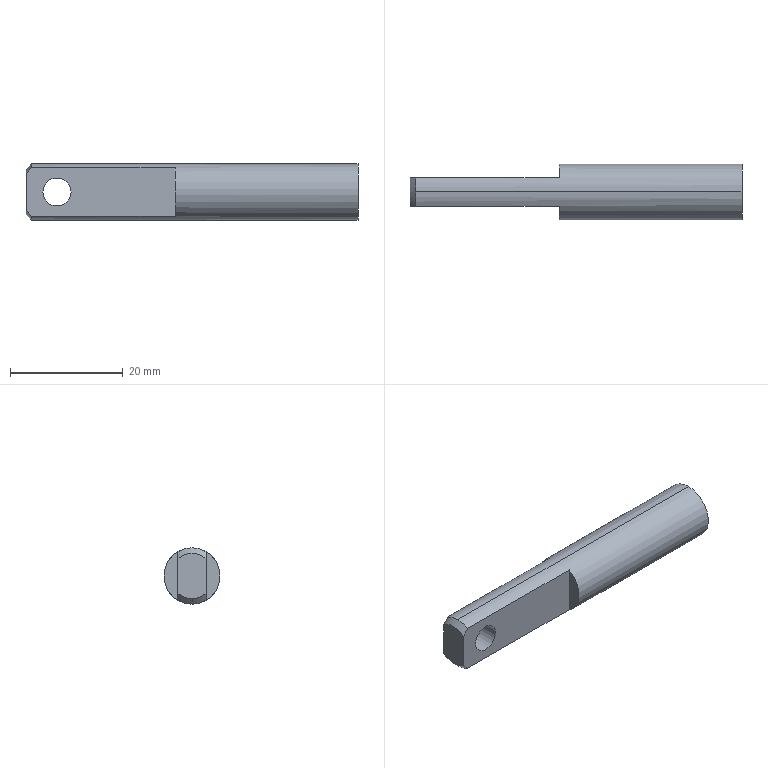Part | STEP file | mandrel_default | 1 solid | 13 faces | box 59 x 10 x 10 mm | volume 3717 mm3 | plane 6 | cylinder 4 | cone 3 | commonest cylinder face diameters 5 x2 10 x2
STEP:
#1=CARTESIAN_POINT('',(0.,0.,0.));
#2=DIRECTION('',(0.,0.,1.));
#3=DIRECTION('',(1.,0.,0.));
#4=AXIS2_PLACEMENT_3D('',#1,#2,#3);
#5=CARTESIAN_POINT('',(-59.,0.,-4.));
#6=VERTEX_POINT('',#5);
#7=CARTESIAN_POINT('',(-59.,-2.5,-3.122));
#8=VERTEX_POINT('',#7);
#9=CARTESIAN_POINT('',(-59.,0.,0.));
#10=DIRECTION('',(-1.,0.,0.));
#11=DIRECTION('',(0.,0.,-1.));
#12=AXIS2_PLACEMENT_3D('',#9,#10,#11);
#13=CIRCLE('',#12,4.);
#14=CARTESIAN_POINT('',(-58.,0.,0.));
#15=DIRECTION('',(1.,0.,0.));
#16=DIRECTION('',(0.,0.,-1.));
#17=AXIS2_PLACEMENT_3D('',#14,#15,#16);
#18=CONICAL_SURFACE('',#17,5.,0.7854);
#19=CARTESIAN_POINT('',(6.283,-1.));
#20=DIRECTION('',(-1.,0.));
#21=VECTOR('',#20,1.);
#22=LINE('',#19,#21);
#23=(GEOMETRIC_REPRESENTATION_CONTEXT(2)PARAMETRIC_REPRESENTATION_CONTEXT()REPRESENTATION_CONTEXT('',''));
#24=DEFINITIONAL_REPRESENTATION('',(#22),#23);
#25=PCURVE('',#18,#24);
#26=CARTESIAN_POINT('',(-59.,0.,0.));
#27=DIRECTION('',(1.,0.,0.));
#28=DIRECTION('',(0.,0.,-1.));
#29=AXIS2_PLACEMENT_3D('',#26,#27,#28);
#30=PLANE('',#29);
#31=CARTESIAN_POINT('',(4.,0.));
#32=CARTESIAN_POINT('',(4.,-6.928));
#33=CARTESIAN_POINT('',(-2.,-3.464));
#34=CARTESIAN_POINT('',(-8.,0.));
#35=CARTESIAN_POINT('',(-2.,3.464));
#36=CARTESIAN_POINT('',(4.,6.928));
#37=CARTESIAN_POINT('',(4.,0.));
#38=(BOUNDED_CURVE()B_SPLINE_CURVE(2,(#31,#32,#33,#34,#35,#36,#37),.UNSPECIFIED.,.T.,.F.)B_SPLINE_CURVE_WITH_KNOTS((1,2,2,2,2,1),(-2.094,0.,2.094,4.189,6.283,8.378),.UNSPECIFIED.)CURVE()GEOMETRIC_REPRESENTATION_ITEM()RATIONAL_B_SPLINE_CURVE((1.,0.5,1.,0.5,1.,0.5,1.))REPRESENTATION_ITEM(''));
#39=(GEOMETRIC_REPRESENTATION_CONTEXT(2)PARAMETRIC_REPRESENTATION_CONTEXT()REPRESENTATION_CONTEXT('',''));
#40=DEFINITIONAL_REPRESENTATION('',(#38),#39);
#41=PCURVE('',#30,#40);
#42=SURFACE_CURVE('',#13,(#25,#41),.PCURVE_S1.);
#43=EDGE_CURVE('',#6,#8,#42,.T.);
#44=ORIENTED_EDGE('',*,*,#43,.F.);
#45=CARTESIAN_POINT('',(-58.,0.,-5.));
#46=VERTEX_POINT('',#45);
#47=CARTESIAN_POINT('',(-58.,0.,-5.));
#48=DIRECTION('',(0.7071,0.,-0.7071));
#49=VECTOR('',#48,1.);
#50=LINE('',#47,#49);
#51=CARTESIAN_POINT('',(6.283,0.));
#52=DIRECTION('',(0.,1.));
#53=VECTOR('',#52,1.);
#54=LINE('',#51,#53);
#55=(GEOMETRIC_REPRESENTATION_CONTEXT(2)PARAMETRIC_REPRESENTATION_CONTEXT()REPRESENTATION_CONTEXT('',''));
#56=DEFINITIONAL_REPRESENTATION('',(#54),#55);
#57=PCURVE('',#18,#56);
#58=CARTESIAN_POINT('',(-58.,0.,0.));
#59=DIRECTION('',(1.,0.,0.));
#60=DIRECTION('',(0.,0.,-1.));
#61=AXIS2_PLACEMENT_3D('',#58,#59,#60);
#62=CONICAL_SURFACE('',#61,5.,0.7854);
#63=CARTESIAN_POINT('',(0.,0.));
#64=DIRECTION('',(0.,1.));
#65=VECTOR('',#64,1.);
#66=LINE('',#63,#65);
#67=(GEOMETRIC_REPRESENTATION_CONTEXT(2)PARAMETRIC_REPRESENTATION_CONTEXT()REPRESENTATION_CONTEXT('',''));
#68=DEFINITIONAL_REPRESENTATION('',(#66),#67);
#69=PCURVE('',#62,#68);
#70=SURFACE_CURVE('',#50,(#57,#69),.PCURVE_S1.);
#71=EDGE_CURVE('',#6,#46,#70,.T.);
#72=ORIENTED_EDGE('',*,*,#71,.T.);
#73=CARTESIAN_POINT('',(-58.,-2.5,-4.33));
#74=VERTEX_POINT('',#73);
#75=CARTESIAN_POINT('',(-58.,0.,0.));
#76=DIRECTION('',(1.,0.,0.));
#77=DIRECTION('',(0.,0.,-1.));
#78=AXIS2_PLACEMENT_3D('',#75,#76,#77);
#79=CIRCLE('',#78,5.);
#80=CARTESIAN_POINT('',(0.,0.));
#81=DIRECTION('',(1.,0.));
#82=VECTOR('',#81,1.);
#83=LINE('',#80,#82);
#84=(GEOMETRIC_REPRESENTATION_CONTEXT(2)PARAMETRIC_REPRESENTATION_CONTEXT()REPRESENTATION_CONTEXT('',''));
#85=DEFINITIONAL_REPRESENTATION('',(#83),#84);
#86=PCURVE('',#18,#85);
#87=CARTESIAN_POINT('',(-59.,0.,0.));
#88=DIRECTION('',(1.,0.,0.));
#89=DIRECTION('',(0.,0.,-1.));
#90=AXIS2_PLACEMENT_3D('',#87,#88,#89);
#91=CYLINDRICAL_SURFACE('',#90,5.);
#92=CARTESIAN_POINT('',(0.,1.));
#93=DIRECTION('',(1.,0.));
#94=VECTOR('',#93,1.);
#95=LINE('',#92,#94);
#96=(GEOMETRIC_REPRESENTATION_CONTEXT(2)PARAMETRIC_REPRESENTATION_CONTEXT()REPRESENTATION_CONTEXT('',''));
#97=DEFINITIONAL_REPRESENTATION('',(#95),#96);
#98=PCURVE('',#91,#97);
#99=SURFACE_CURVE('',#79,(#86,#98),.PCURVE_S1.);
#100=EDGE_CURVE('',#74,#46,#99,.T.);
#101=ORIENTED_EDGE('',*,*,#100,.F.);
#102=CARTESIAN_POINT('',(-59.,-2.5,-3.122));
#103=CARTESIAN_POINT('',(-58.678,-2.5,-3.535));
#104=CARTESIAN_POINT('',(-58.342,-2.5,-3.935));
#105=CARTESIAN_POINT('',(-58.,-2.5,-4.33));
#106=B_SPLINE_CURVE_WITH_KNOTS('',3,(#102,#103,#104,#105),.UNSPECIFIED.,.F.,.F.,(4,4),(0.,0.001568),.PIECEWISE_BEZIER_KNOTS.);
#107=CARTESIAN_POINT('',(5.608,-1.));
#108=CARTESIAN_POINT('',(5.611,-0.9854));
#109=CARTESIAN_POINT('',(5.617,-0.9561));
#110=CARTESIAN_POINT('',(5.625,-0.9119));
#111=CARTESIAN_POINT('',(5.633,-0.8676));
#112=CARTESIAN_POINT('',(5.642,-0.8231));
#113=CARTESIAN_POINT('',(5.649,-0.7785));
#114=CARTESIAN_POINT('',(5.657,-0.7337));
#115=CARTESIAN_POINT('',(5.665,-0.6887));
#116=CARTESIAN_POINT('',(5.672,-0.6437));
#117=CARTESIAN_POINT('',(5.679,-0.5984));
#118=CARTESIAN_POINT('',(5.686,-0.5531));
#119=CARTESIAN_POINT('',(5.693,-0.5076));
#120=CARTESIAN_POINT('',(5.7,-0.462));
#121=CARTESIAN_POINT('',(5.706,-0.4163));
#122=CARTESIAN_POINT('',(5.713,-0.3704));
#123=CARTESIAN_POINT('',(5.719,-0.3245));
#124=CARTESIAN_POINT('',(5.725,-0.2784));
#125=CARTESIAN_POINT('',(5.731,-0.2322));
#126=CARTESIAN_POINT('',(5.737,-0.186));
#127=CARTESIAN_POINT('',(5.743,-0.1396));
#128=CARTESIAN_POINT('',(5.749,-0.09318));
#129=CARTESIAN_POINT('',(5.754,-0.04664));
#130=CARTESIAN_POINT('',(5.758,-0.01556));
#131=CARTESIAN_POINT('',(5.76,0.));
#132=B_SPLINE_CURVE_WITH_KNOTS('',3,(#107,#108,#109,#110,#111,#112,#113,#114,#115,#116,#117,#118,#119,#120,#121,#122,#123,#124,#125,#126,#127,#128,#129,#130,#131),.UNSPECIFIED.,.F.,.F.,(4,1,1,1,1,1,1,1,1,1,1,1,1,1,1,1,1,1,1,1,1,1,4),(0.,0.00007127,0.0001425,0.0002138,0.0002851,0.0003563,0.0004276,0.0004989,0.0005702,0.0006414,0.0007127,0.000784,0.0008552,0.0009265,0.0009978,0.001069,0.00114,0.001212,0.001283,0.001354,0.001425,0.001497,0.001568),.QUASI_UNIFORM_KNOTS.);
#133=(GEOMETRIC_REPRESENTATION_CONTEXT(2)PARAMETRIC_REPRESENTATION_CONTEXT()REPRESENTATION_CONTEXT('',''));
#134=DEFINITIONAL_REPRESENTATION('',(#132),#133);
#135=PCURVE('',#18,#134);
#136=CARTESIAN_POINT('',(-64.008,-2.5,-5.));
#137=DIRECTION('',(0.,1.,0.));
#138=DIRECTION('',(-1.,0.,0.));
#139=AXIS2_PLACEMENT_3D('',#136,#137,#138);
#140=PLANE('',#139);
#141=CARTESIAN_POINT('',(-5.008,1.878));
#142=CARTESIAN_POINT('',(-5.33,1.465));
#143=CARTESIAN_POINT('',(-5.666,1.065));
#144=CARTESIAN_POINT('',(-6.008,0.6699));
#145=B_SPLINE_CURVE_WITH_KNOTS('',3,(#141,#142,#143,#144),.UNSPECIFIED.,.F.,.F.,(4,4),(0.,0.001568),.PIECEWISE_BEZIER_KNOTS.);
#146=(GEOMETRIC_REPRESENTATION_CONTEXT(2)PARAMETRIC_REPRESENTATION_CONTEXT()REPRESENTATION_CONTEXT('',''));
#147=DEFINITIONAL_REPRESENTATION('',(#145),#146);
#148=PCURVE('',#140,#147);
#149=SURFACE_CURVE('',#106,(#135,#148),.PCURVE_S1.);
#150=EDGE_CURVE('',#8,#74,#149,.T.);
#151=ORIENTED_EDGE('',*,*,#150,.F.);
#152=EDGE_LOOP('',(#44,#72,#101,#151));
#153=FACE_BOUND('',#152,.T.);
#154=ADVANCED_FACE('',(#153),#18,.T.);
#155=CARTESIAN_POINT('',(-56.,-2.5,0.));
#156=VERTEX_POINT('',#155);
#157=CARTESIAN_POINT('',(-56.,2.5,0.));
#158=VERTEX_POINT('',#157);
#159=CARTESIAN_POINT('',(-56.,-5.,0.));
#160=DIRECTION('',(0.,1.,0.));
#161=VECTOR('',#160,1.);
#162=LINE('',#159,#161);
#163=CARTESIAN_POINT('',(-53.5,-5.,0.));
#164=DIRECTION('',(0.,1.,0.));
#165=DIRECTION('',(-1.,0.,0.));
#166=AXIS2_PLACEMENT_3D('',#163,#164,#165);
#167=CYLINDRICAL_SURFACE('',#166,2.5);
#168=CARTESIAN_POINT('',(6.283,0.));
#169=DIRECTION('',(0.,1.));
#170=VECTOR('',#169,1.);
#171=LINE('',#168,#170);
#172=(GEOMETRIC_REPRESENTATION_CONTEXT(2)PARAMETRIC_REPRESENTATION_CONTEXT()REPRESENTATION_CONTEXT('',''));
#173=DEFINITIONAL_REPRESENTATION('',(#171),#172);
#174=PCURVE('',#167,#173);
#175=CARTESIAN_POINT('',(-53.5,-5.,0.));
#176=DIRECTION('',(0.,1.,0.));
#177=DIRECTION('',(-1.,0.,0.));
#178=AXIS2_PLACEMENT_3D('',#175,#176,#177);
#179=CYLINDRICAL_SURFACE('',#178,2.5);
#180=CARTESIAN_POINT('',(0.,0.));
#181=DIRECTION('',(0.,1.));
#182=VECTOR('',#181,1.);
#183=LINE('',#180,#182);
#184=(GEOMETRIC_REPRESENTATION_CONTEXT(2)PARAMETRIC_REPRESENTATION_CONTEXT()REPRESENTATION_CONTEXT('',''));
#185=DEFINITIONAL_REPRESENTATION('',(#183),#184);
#186=PCURVE('',#179,#185);
#187=SURFACE_CURVE('',#162,(#174,#186),.PCURVE_S1.);
#188=EDGE_CURVE('',#156,#158,#187,.T.);
#189=ORIENTED_EDGE('',*,*,#188,.T.);
#190=CARTESIAN_POINT('',(-51.,2.5,0.));
#191=VERTEX_POINT('',#190);
#192=CARTESIAN_POINT('',(-53.5,2.5,0.));
#193=DIRECTION('',(0.,1.,0.));
#194=DIRECTION('',(-1.,0.,0.));
#195=AXIS2_PLACEMENT_3D('',#192,#193,#194);
#196=CIRCLE('',#195,2.5);
#197=CARTESIAN_POINT('',(0.,7.5));
#198=DIRECTION('',(1.,0.));
#199=VECTOR('',#198,1.);
#200=LINE('',#197,#199);
#201=(GEOMETRIC_REPRESENTATION_CONTEXT(2)PARAMETRIC_REPRESENTATION_CONTEXT()REPRESENTATION_CONTEXT('',''));
#202=DEFINITIONAL_REPRESENTATION('',(#200),#201);
#203=PCURVE('',#167,#202);
#204=CARTESIAN_POINT('',(-61.463,2.5,-5.));
#205=DIRECTION('',(0.,-1.,0.));
#206=DIRECTION('',(1.,0.,0.));
#207=AXIS2_PLACEMENT_3D('',#204,#205,#206);
#208=PLANE('',#207);
#209=CARTESIAN_POINT('',(5.463,5.));
#210=CARTESIAN_POINT('',(5.463,9.33));
#211=CARTESIAN_POINT('',(9.213,7.165));
#212=CARTESIAN_POINT('',(12.963,5.));
#213=CARTESIAN_POINT('',(9.213,2.835));
#214=CARTESIAN_POINT('',(5.463,0.6699));
#215=CARTESIAN_POINT('',(5.463,5.));
#216=(BOUNDED_CURVE()B_SPLINE_CURVE(2,(#209,#210,#211,#212,#213,#214,#215),.UNSPECIFIED.,.T.,.F.)B_SPLINE_CURVE_WITH_KNOTS((1,2,2,2,2,1),(-2.094,0.,2.094,4.189,6.283,8.378),.UNSPECIFIED.)CURVE()GEOMETRIC_REPRESENTATION_ITEM()RATIONAL_B_SPLINE_CURVE((1.,0.5,1.,0.5,1.,0.5,1.))REPRESENTATION_ITEM(''));
#217=(GEOMETRIC_REPRESENTATION_CONTEXT(2)PARAMETRIC_REPRESENTATION_CONTEXT()REPRESENTATION_CONTEXT('',''));
#218=DEFINITIONAL_REPRESENTATION('',(#216),#217);
#219=PCURVE('',#208,#218);
#220=SURFACE_CURVE('',#196,(#203,#219),.PCURVE_S1.);
#221=EDGE_CURVE('',#191,#158,#220,.T.);
#222=ORIENTED_EDGE('',*,*,#221,.F.);
#223=CARTESIAN_POINT('',(-51.,-2.5,0.));
#224=VERTEX_POINT('',#223);
#225=CARTESIAN_POINT('',(-51.,-5.,0.));
#226=DIRECTION('',(0.,1.,0.));
#227=VECTOR('',#226,1.);
#228=LINE('',#225,#227);
#229=CARTESIAN_POINT('',(3.142,0.));
#230=DIRECTION('',(0.,1.));
#231=VECTOR('',#230,1.);
#232=LINE('',#229,#231);
#233=(GEOMETRIC_REPRESENTATION_CONTEXT(2)PARAMETRIC_REPRESENTATION_CONTEXT()REPRESENTATION_CONTEXT('',''));
#234=DEFINITIONAL_REPRESENTATION('',(#232),#233);
#235=PCURVE('',#167,#234);
#236=CARTESIAN_POINT('',(3.142,0.));
#237=DIRECTION('',(0.,1.));
#238=VECTOR('',#237,1.);
#239=LINE('',#236,#238);
#240=(GEOMETRIC_REPRESENTATION_CONTEXT(2)PARAMETRIC_REPRESENTATION_CONTEXT()REPRESENTATION_CONTEXT('',''));
#241=DEFINITIONAL_REPRESENTATION('',(#239),#240);
#242=PCURVE('',#179,#241);
#243=SURFACE_CURVE('',#228,(#235,#242),.PCURVE_S1.);
#244=EDGE_CURVE('',#224,#191,#243,.T.);
#245=ORIENTED_EDGE('',*,*,#244,.F.);
#246=CARTESIAN_POINT('',(-53.5,-2.5,0.));
#247=DIRECTION('',(0.,1.,0.));
#248=DIRECTION('',(-1.,0.,0.));
#249=AXIS2_PLACEMENT_3D('',#246,#247,#248);
#250=CIRCLE('',#249,2.5);
#251=CARTESIAN_POINT('',(0.,2.5));
#252=DIRECTION('',(1.,0.));
#253=VECTOR('',#252,1.);
#254=LINE('',#251,#253);
#255=(GEOMETRIC_REPRESENTATION_CONTEXT(2)PARAMETRIC_REPRESENTATION_CONTEXT()REPRESENTATION_CONTEXT('',''));
#256=DEFINITIONAL_REPRESENTATION('',(#254),#255);
#257=PCURVE('',#167,#256);
#258=CARTESIAN_POINT('',(-10.508,5.));
#259=DIRECTION('',(1.,0.));
#260=AXIS2_PLACEMENT_2D('',#258,#259);
#261=CIRCLE('',#260,2.5);
#262=(GEOMETRIC_REPRESENTATION_CONTEXT(2)PARAMETRIC_REPRESENTATION_CONTEXT()REPRESENTATION_CONTEXT('',''));
#263=DEFINITIONAL_REPRESENTATION('',(#261),#262);
#264=PCURVE('',#140,#263);
#265=SURFACE_CURVE('',#250,(#257,#264),.PCURVE_S1.);
#266=EDGE_CURVE('',#224,#156,#265,.T.);
#267=ORIENTED_EDGE('',*,*,#266,.T.);
#268=EDGE_LOOP('',(#189,#222,#245,#267));
#269=FACE_BOUND('',#268,.F.);
#270=ADVANCED_FACE('',(#269),#167,.F.);
#271=CARTESIAN_POINT('',(-58.,2.5,4.33));
#272=VERTEX_POINT('',#271);
#273=CARTESIAN_POINT('',(-58.,0.,5.));
#274=VERTEX_POINT('',#273);
#275=CARTESIAN_POINT('',(-58.,0.,0.));
#276=DIRECTION('',(1.,0.,0.));
#277=DIRECTION('',(0.,0.,-1.));
#278=AXIS2_PLACEMENT_3D('',#275,#276,#277);
#279=CIRCLE('',#278,5.);
#280=CARTESIAN_POINT('',(-59.,0.,0.));
#281=DIRECTION('',(1.,0.,0.));
#282=DIRECTION('',(0.,0.,-1.));
#283=AXIS2_PLACEMENT_3D('',#280,#281,#282);
#284=CYLINDRICAL_SURFACE('',#283,5.);
#285=CARTESIAN_POINT('',(0.,1.));
#286=DIRECTION('',(1.,0.));
#287=VECTOR('',#286,1.);
#288=LINE('',#285,#287);
#289=(GEOMETRIC_REPRESENTATION_CONTEXT(2)PARAMETRIC_REPRESENTATION_CONTEXT()REPRESENTATION_CONTEXT('',''));
#290=DEFINITIONAL_REPRESENTATION('',(#288),#289);
#291=PCURVE('',#284,#290);
#292=CARTESIAN_POINT('',(-58.,0.,0.));
#293=DIRECTION('',(1.,0.,0.));
#294=DIRECTION('',(0.,0.,-1.));
#295=AXIS2_PLACEMENT_3D('',#292,#293,#294);
#296=CONICAL_SURFACE('',#295,5.,0.7854);
#297=CARTESIAN_POINT('',(0.,0.));
#298=DIRECTION('',(1.,0.));
#299=VECTOR('',#298,1.);
#300=LINE('',#297,#299);
#301=(GEOMETRIC_REPRESENTATION_CONTEXT(2)PARAMETRIC_REPRESENTATION_CONTEXT()REPRESENTATION_CONTEXT('',''));
#302=DEFINITIONAL_REPRESENTATION('',(#300),#301);
#303=PCURVE('',#296,#302);
#304=SURFACE_CURVE('',#279,(#291,#303),.PCURVE_S1.);
#305=EDGE_CURVE('',#272,#274,#304,.T.);
#306=ORIENTED_EDGE('',*,*,#305,.T.);
#307=CARTESIAN_POINT('',(0.,0.,5.));
#308=VERTEX_POINT('',#307);
#309=CARTESIAN_POINT('',(-59.,0.,5.));
#310=DIRECTION('',(1.,0.,0.));
#311=VECTOR('',#310,1.);
#312=LINE('',#309,#311);
#313=CARTESIAN_POINT('',(3.142,0.));
#314=DIRECTION('',(0.,1.));
#315=VECTOR('',#314,1.);
#316=LINE('',#313,#315);
#317=(GEOMETRIC_REPRESENTATION_CONTEXT(2)PARAMETRIC_REPRESENTATION_CONTEXT()REPRESENTATION_CONTEXT('',''));
#318=DEFINITIONAL_REPRESENTATION('',(#316),#317);
#319=PCURVE('',#284,#318);
#320=CARTESIAN_POINT('',(3.142,0.));
#321=DIRECTION('',(0.,1.));
#322=VECTOR('',#321,1.);
#323=LINE('',#320,#322);
#324=(GEOMETRIC_REPRESENTATION_CONTEXT(2)PARAMETRIC_REPRESENTATION_CONTEXT()REPRESENTATION_CONTEXT('',''));
#325=DEFINITIONAL_REPRESENTATION('',(#323),#324);
#326=PCURVE('',#91,#325);
#327=SURFACE_CURVE('',#312,(#319,#326),.PCURVE_S1.);
#328=EDGE_CURVE('',#274,#308,#327,.T.);
#329=ORIENTED_EDGE('',*,*,#328,.T.);
#330=CARTESIAN_POINT('',(0.,0.,-5.));
#331=VERTEX_POINT('',#330);
#332=CARTESIAN_POINT('',(0.,0.,0.));
#333=DIRECTION('',(1.,0.,0.));
#334=DIRECTION('',(0.,0.,-1.));
#335=AXIS2_PLACEMENT_3D('',#332,#333,#334);
#336=CIRCLE('',#335,5.);
#337=CARTESIAN_POINT('',(0.,59.));
#338=DIRECTION('',(1.,0.));
#339=VECTOR('',#338,1.);
#340=LINE('',#337,#339);
#341=(GEOMETRIC_REPRESENTATION_CONTEXT(2)PARAMETRIC_REPRESENTATION_CONTEXT()REPRESENTATION_CONTEXT('',''));
#342=DEFINITIONAL_REPRESENTATION('',(#340),#341);
#343=PCURVE('',#284,#342);
#344=CARTESIAN_POINT('',(0.,0.,0.));
#345=DIRECTION('',(1.,0.,0.));
#346=DIRECTION('',(0.,0.,-1.));
#347=AXIS2_PLACEMENT_3D('',#344,#345,#346);
#348=PLANE('',#347);
#349=CARTESIAN_POINT('',(0.,0.));
#350=DIRECTION('',(1.,0.));
#351=AXIS2_PLACEMENT_2D('',#349,#350);
#352=CIRCLE('',#351,5.);
#353=(GEOMETRIC_REPRESENTATION_CONTEXT(2)PARAMETRIC_REPRESENTATION_CONTEXT()REPRESENTATION_CONTEXT('',''));
#354=DEFINITIONAL_REPRESENTATION('',(#352),#353);
#355=PCURVE('',#348,#354);
#356=SURFACE_CURVE('',#336,(#343,#355),.PCURVE_S1.);
#357=EDGE_CURVE('',#331,#308,#356,.T.);
#358=ORIENTED_EDGE('',*,*,#357,.F.);
#359=CARTESIAN_POINT('',(-59.,0.,-5.));
#360=DIRECTION('',(1.,0.,0.));
#361=VECTOR('',#360,1.);
#362=LINE('',#359,#361);
#363=CARTESIAN_POINT('',(0.,0.));
#364=DIRECTION('',(0.,1.));
#365=VECTOR('',#364,1.);
#366=LINE('',#363,#365);
#367=(GEOMETRIC_REPRESENTATION_CONTEXT(2)PARAMETRIC_REPRESENTATION_CONTEXT()REPRESENTATION_CONTEXT('',''));
#368=DEFINITIONAL_REPRESENTATION('',(#366),#367);
#369=PCURVE('',#284,#368);
#370=CARTESIAN_POINT('',(6.283,0.));
#371=DIRECTION('',(0.,1.));
#372=VECTOR('',#371,1.);
#373=LINE('',#370,#372);
#374=(GEOMETRIC_REPRESENTATION_CONTEXT(2)PARAMETRIC_REPRESENTATION_CONTEXT()REPRESENTATION_CONTEXT('',''));
#375=DEFINITIONAL_REPRESENTATION('',(#373),#374);
#376=PCURVE('',#91,#375);
#377=SURFACE_CURVE('',#362,(#369,#376),.PCURVE_S1.);
#378=EDGE_CURVE('',#46,#331,#377,.T.);
#379=ORIENTED_EDGE('',*,*,#378,.F.);
#380=CARTESIAN_POINT('',(-58.,2.5,-4.33));
#381=VERTEX_POINT('',#380);
#382=CARTESIAN_POINT('',(-58.,0.,0.));
#383=DIRECTION('',(1.,0.,0.));
#384=DIRECTION('',(0.,0.,-1.));
#385=AXIS2_PLACEMENT_3D('',#382,#383,#384);
#386=CIRCLE('',#385,5.);
#387=CARTESIAN_POINT('',(0.,1.));
#388=DIRECTION('',(1.,0.));
#389=VECTOR('',#388,1.);
#390=LINE('',#387,#389);
#391=(GEOMETRIC_REPRESENTATION_CONTEXT(2)PARAMETRIC_REPRESENTATION_CONTEXT()REPRESENTATION_CONTEXT('',''));
#392=DEFINITIONAL_REPRESENTATION('',(#390),#391);
#393=PCURVE('',#284,#392);
#394=CARTESIAN_POINT('',(0.,0.));
#395=DIRECTION('',(1.,0.));
#396=VECTOR('',#395,1.);
#397=LINE('',#394,#396);
#398=(GEOMETRIC_REPRESENTATION_CONTEXT(2)PARAMETRIC_REPRESENTATION_CONTEXT()REPRESENTATION_CONTEXT('',''));
#399=DEFINITIONAL_REPRESENTATION('',(#397),#398);
#400=PCURVE('',#62,#399);
#401=SURFACE_CURVE('',#386,(#393,#400),.PCURVE_S1.);
#402=EDGE_CURVE('',#46,#381,#401,.T.);
#403=ORIENTED_EDGE('',*,*,#402,.T.);
#404=CARTESIAN_POINT('',(-32.5,2.5,-4.33));
#405=VERTEX_POINT('',#404);
#406=CARTESIAN_POINT('',(-59.,2.5,-4.33));
#407=DIRECTION('',(-1.,0.,0.));
#408=VECTOR('',#407,1.);
#409=LINE('',#406,#408);
#410=CARTESIAN_POINT('',(0.5236,0.));
#411=DIRECTION('',(0.,-1.));
#412=VECTOR('',#411,1.);
#413=LINE('',#410,#412);
#414=(GEOMETRIC_REPRESENTATION_CONTEXT(2)PARAMETRIC_REPRESENTATION_CONTEXT()REPRESENTATION_CONTEXT('',''));
#415=DEFINITIONAL_REPRESENTATION('',(#413),#414);
#416=PCURVE('',#284,#415);
#417=CARTESIAN_POINT('',(2.463,0.6699));
#418=DIRECTION('',(-1.,0.));
#419=VECTOR('',#418,1.);
#420=LINE('',#417,#419);
#421=(GEOMETRIC_REPRESENTATION_CONTEXT(2)PARAMETRIC_REPRESENTATION_CONTEXT()REPRESENTATION_CONTEXT('',''));
#422=DEFINITIONAL_REPRESENTATION('',(#420),#421);
#423=PCURVE('',#208,#422);
#424=SURFACE_CURVE('',#409,(#416,#423),.PCURVE_S1.);
#425=EDGE_CURVE('',#405,#381,#424,.T.);
#426=ORIENTED_EDGE('',*,*,#425,.F.);
#427=CARTESIAN_POINT('',(-32.5,2.5,4.33));
#428=VERTEX_POINT('',#427);
#429=CARTESIAN_POINT('',(-32.5,0.,0.));
#430=DIRECTION('',(-1.,0.,0.));
#431=DIRECTION('',(0.,0.,-1.));
#432=AXIS2_PLACEMENT_3D('',#429,#430,#431);
#433=CIRCLE('',#432,5.);
#434=CARTESIAN_POINT('',(6.283,26.5));
#435=DIRECTION('',(-1.,0.));
#436=VECTOR('',#435,1.);
#437=LINE('',#434,#436);
#438=(GEOMETRIC_REPRESENTATION_CONTEXT(2)PARAMETRIC_REPRESENTATION_CONTEXT()REPRESENTATION_CONTEXT('',''));
#439=DEFINITIONAL_REPRESENTATION('',(#437),#438);
#440=PCURVE('',#284,#439);
#441=CARTESIAN_POINT('',(-32.5,7.127,-5.));
#442=DIRECTION('',(1.,0.,0.));
#443=DIRECTION('',(0.,0.,-1.));
#444=AXIS2_PLACEMENT_3D('',#441,#442,#443);
#445=PLANE('',#444);
#446=CARTESIAN_POINT('',(0.,-7.127));
#447=CARTESIAN_POINT('',(0.,-15.787));
#448=CARTESIAN_POINT('',(-7.5,-11.457));
#449=CARTESIAN_POINT('',(-15.,-7.127));
#450=CARTESIAN_POINT('',(-7.5,-2.797));
#451=CARTESIAN_POINT('',(0.,1.533));
#452=CARTESIAN_POINT('',(0.,-7.127));
#453=(BOUNDED_CURVE()B_SPLINE_CURVE(2,(#446,#447,#448,#449,#450,#451,#452),.UNSPECIFIED.,.T.,.F.)B_SPLINE_CURVE_WITH_KNOTS((1,2,2,2,2,1),(-2.094,0.,2.094,4.189,6.283,8.378),.UNSPECIFIED.)CURVE()GEOMETRIC_REPRESENTATION_ITEM()RATIONAL_B_SPLINE_CURVE((1.,0.5,1.,0.5,1.,0.5,1.))REPRESENTATION_ITEM(''));
#454=(GEOMETRIC_REPRESENTATION_CONTEXT(2)PARAMETRIC_REPRESENTATION_CONTEXT()REPRESENTATION_CONTEXT('',''));
#455=DEFINITIONAL_REPRESENTATION('',(#453),#454);
#456=PCURVE('',#445,#455);
#457=SURFACE_CURVE('',#433,(#440,#456),.PCURVE_S1.);
#458=EDGE_CURVE('',#428,#405,#457,.T.);
#459=ORIENTED_EDGE('',*,*,#458,.F.);
#460=CARTESIAN_POINT('',(-59.,2.5,4.33));
#461=DIRECTION('',(1.,0.,0.));
#462=VECTOR('',#461,1.);
#463=LINE('',#460,#462);
#464=CARTESIAN_POINT('',(2.618,0.));
#465=DIRECTION('',(0.,1.));
#466=VECTOR('',#465,1.);
#467=LINE('',#464,#466);
#468=(GEOMETRIC_REPRESENTATION_CONTEXT(2)PARAMETRIC_REPRESENTATION_CONTEXT()REPRESENTATION_CONTEXT('',''));
#469=DEFINITIONAL_REPRESENTATION('',(#467),#468);
#470=PCURVE('',#284,#469);
#471=CARTESIAN_POINT('',(2.463,9.33));
#472=DIRECTION('',(1.,0.));
#473=VECTOR('',#472,1.);
#474=LINE('',#471,#473);
#475=(GEOMETRIC_REPRESENTATION_CONTEXT(2)PARAMETRIC_REPRESENTATION_CONTEXT()REPRESENTATION_CONTEXT('',''));
#476=DEFINITIONAL_REPRESENTATION('',(#474),#475);
#477=PCURVE('',#208,#476);
#478=SURFACE_CURVE('',#463,(#470,#477),.PCURVE_S1.);
#479=EDGE_CURVE('',#272,#428,#478,.T.);
#480=ORIENTED_EDGE('',*,*,#479,.F.);
#481=EDGE_LOOP('',(#306,#329,#358,#379,#403,#426,#459,#480));
#482=FACE_BOUND('',#481,.T.);
#483=ADVANCED_FACE('',(#482),#284,.T.);
#484=ORIENTED_EDGE('',*,*,#328,.F.);
#485=CARTESIAN_POINT('',(-58.,-2.5,4.33));
#486=VERTEX_POINT('',#485);
#487=CARTESIAN_POINT('',(-58.,0.,0.));
#488=DIRECTION('',(1.,0.,0.));
#489=DIRECTION('',(0.,0.,-1.));
#490=AXIS2_PLACEMENT_3D('',#487,#488,#489);
#491=CIRCLE('',#490,5.);
#492=CARTESIAN_POINT('',(0.,1.));
#493=DIRECTION('',(1.,0.));
#494=VECTOR('',#493,1.);
#495=LINE('',#492,#494);
#496=(GEOMETRIC_REPRESENTATION_CONTEXT(2)PARAMETRIC_REPRESENTATION_CONTEXT()REPRESENTATION_CONTEXT('',''));
#497=DEFINITIONAL_REPRESENTATION('',(#495),#496);
#498=PCURVE('',#91,#497);
#499=CARTESIAN_POINT('',(0.,0.));
#500=DIRECTION('',(1.,0.));
#501=VECTOR('',#500,1.);
#502=LINE('',#499,#501);
#503=(GEOMETRIC_REPRESENTATION_CONTEXT(2)PARAMETRIC_REPRESENTATION_CONTEXT()REPRESENTATION_CONTEXT('',''));
#504=DEFINITIONAL_REPRESENTATION('',(#502),#503);
#505=PCURVE('',#296,#504);
#506=SURFACE_CURVE('',#491,(#498,#505),.PCURVE_S1.);
#507=EDGE_CURVE('',#274,#486,#506,.T.);
#508=ORIENTED_EDGE('',*,*,#507,.T.);
#509=CARTESIAN_POINT('',(-32.5,-2.5,4.33));
#510=VERTEX_POINT('',#509);
#511=CARTESIAN_POINT('',(-59.,-2.5,4.33));
#512=DIRECTION('',(-1.,0.,0.));
#513=VECTOR('',#512,1.);
#514=LINE('',#511,#513);
#515=CARTESIAN_POINT('',(3.665,0.));
#516=DIRECTION('',(0.,-1.));
#517=VECTOR('',#516,1.);
#518=LINE('',#515,#517);
#519=(GEOMETRIC_REPRESENTATION_CONTEXT(2)PARAMETRIC_REPRESENTATION_CONTEXT()REPRESENTATION_CONTEXT('',''));
#520=DEFINITIONAL_REPRESENTATION('',(#518),#519);
#521=PCURVE('',#91,#520);
#522=CARTESIAN_POINT('',(-5.008,9.33));
#523=DIRECTION('',(1.,0.));
#524=VECTOR('',#523,1.);
#525=LINE('',#522,#524);
#526=(GEOMETRIC_REPRESENTATION_CONTEXT(2)PARAMETRIC_REPRESENTATION_CONTEXT()REPRESENTATION_CONTEXT('',''));
#527=DEFINITIONAL_REPRESENTATION('',(#525),#526);
#528=PCURVE('',#140,#527);
#529=SURFACE_CURVE('',#514,(#521,#528),.PCURVE_S1.);
#530=EDGE_CURVE('',#510,#486,#529,.T.);
#531=ORIENTED_EDGE('',*,*,#530,.F.);
#532=CARTESIAN_POINT('',(-32.5,-2.5,-4.33));
#533=VERTEX_POINT('',#532);
#534=CARTESIAN_POINT('',(-32.5,0.,0.));
#535=DIRECTION('',(-1.,0.,0.));
#536=DIRECTION('',(0.,0.,-1.));
#537=AXIS2_PLACEMENT_3D('',#534,#535,#536);
#538=CIRCLE('',#537,5.);
#539=CARTESIAN_POINT('',(6.283,26.5));
#540=DIRECTION('',(-1.,0.));
#541=VECTOR('',#540,1.);
#542=LINE('',#539,#541);
#543=(GEOMETRIC_REPRESENTATION_CONTEXT(2)PARAMETRIC_REPRESENTATION_CONTEXT()REPRESENTATION_CONTEXT('',''));
#544=DEFINITIONAL_REPRESENTATION('',(#542),#543);
#545=PCURVE('',#91,#544);
#546=CARTESIAN_POINT('',(-32.5,-2.5,-5.));
#547=DIRECTION('',(1.,0.,0.));
#548=DIRECTION('',(0.,0.,-1.));
#549=AXIS2_PLACEMENT_3D('',#546,#547,#548);
#550=PLANE('',#549);
#551=CARTESIAN_POINT('',(0.,2.5));
#552=CARTESIAN_POINT('',(0.,-6.16));
#553=CARTESIAN_POINT('',(-7.5,-1.83));
#554=CARTESIAN_POINT('',(-15.,2.5));
#555=CARTESIAN_POINT('',(-7.5,6.83));
#556=CARTESIAN_POINT('',(0.,11.16));
#557=CARTESIAN_POINT('',(0.,2.5));
#558=(BOUNDED_CURVE()B_SPLINE_CURVE(2,(#551,#552,#553,#554,#555,#556,#557),.UNSPECIFIED.,.T.,.F.)B_SPLINE_CURVE_WITH_KNOTS((1,2,2,2,2,1),(-2.094,0.,2.094,4.189,6.283,8.378),.UNSPECIFIED.)CURVE()GEOMETRIC_REPRESENTATION_ITEM()RATIONAL_B_SPLINE_CURVE((1.,0.5,1.,0.5,1.,0.5,1.))REPRESENTATION_ITEM(''));
#559=(GEOMETRIC_REPRESENTATION_CONTEXT(2)PARAMETRIC_REPRESENTATION_CONTEXT()REPRESENTATION_CONTEXT('',''));
#560=DEFINITIONAL_REPRESENTATION('',(#558),#559);
#561=PCURVE('',#550,#560);
#562=SURFACE_CURVE('',#538,(#545,#561),.PCURVE_S1.);
#563=EDGE_CURVE('',#533,#510,#562,.T.);
#564=ORIENTED_EDGE('',*,*,#563,.F.);
#565=CARTESIAN_POINT('',(-59.,-2.5,-4.33));
#566=DIRECTION('',(1.,0.,0.));
#567=VECTOR('',#566,1.);
#568=LINE('',#565,#567);
#569=CARTESIAN_POINT('',(5.76,0.));
#570=DIRECTION('',(0.,1.));
#571=VECTOR('',#570,1.);
#572=LINE('',#569,#571);
#573=(GEOMETRIC_REPRESENTATION_CONTEXT(2)PARAMETRIC_REPRESENTATION_CONTEXT()REPRESENTATION_CONTEXT('',''));
#574=DEFINITIONAL_REPRESENTATION('',(#572),#573);
#575=PCURVE('',#91,#574);
#576=CARTESIAN_POINT('',(-5.008,0.6699));
#577=DIRECTION('',(-1.,0.));
#578=VECTOR('',#577,1.);
#579=LINE('',#576,#578);
#580=(GEOMETRIC_REPRESENTATION_CONTEXT(2)PARAMETRIC_REPRESENTATION_CONTEXT()REPRESENTATION_CONTEXT('',''));
#581=DEFINITIONAL_REPRESENTATION('',(#579),#580);
#582=PCURVE('',#140,#581);
#583=SURFACE_CURVE('',#568,(#575,#582),.PCURVE_S1.);
#584=EDGE_CURVE('',#74,#533,#583,.T.);
#585=ORIENTED_EDGE('',*,*,#584,.F.);
#586=ORIENTED_EDGE('',*,*,#100,.T.);
#587=ORIENTED_EDGE('',*,*,#378,.T.);
#588=CARTESIAN_POINT('',(0.,0.,0.));
#589=DIRECTION('',(1.,0.,0.));
#590=DIRECTION('',(0.,0.,-1.));
#591=AXIS2_PLACEMENT_3D('',#588,#589,#590);
#592=CIRCLE('',#591,5.);
#593=CARTESIAN_POINT('',(0.,59.));
#594=DIRECTION('',(1.,0.));
#595=VECTOR('',#594,1.);
#596=LINE('',#593,#595);
#597=(GEOMETRIC_REPRESENTATION_CONTEXT(2)PARAMETRIC_REPRESENTATION_CONTEXT()REPRESENTATION_CONTEXT('',''));
#598=DEFINITIONAL_REPRESENTATION('',(#596),#597);
#599=PCURVE('',#91,#598);
#600=CARTESIAN_POINT('',(0.,0.));
#601=DIRECTION('',(1.,0.));
#602=AXIS2_PLACEMENT_2D('',#600,#601);
#603=CIRCLE('',#602,5.);
#604=(GEOMETRIC_REPRESENTATION_CONTEXT(2)PARAMETRIC_REPRESENTATION_CONTEXT()REPRESENTATION_CONTEXT('',''));
#605=DEFINITIONAL_REPRESENTATION('',(#603),#604);
#606=PCURVE('',#348,#605);
#607=SURFACE_CURVE('',#592,(#599,#606),.PCURVE_S1.);
#608=EDGE_CURVE('',#308,#331,#607,.T.);
#609=ORIENTED_EDGE('',*,*,#608,.F.);
#610=EDGE_LOOP('',(#484,#508,#531,#564,#585,#586,#587,#609));
#611=FACE_BOUND('',#610,.T.);
#612=ADVANCED_FACE('',(#611),#91,.T.);
#613=CARTESIAN_POINT('',(-59.,2.5,3.122));
#614=VERTEX_POINT('',#613);
#615=CARTESIAN_POINT('',(-59.,2.5,-3.122));
#616=VERTEX_POINT('',#615);
#617=CARTESIAN_POINT('',(-59.,2.5,0.));
#618=DIRECTION('',(0.,0.,-1.));
#619=VECTOR('',#618,1.);
#620=LINE('',#617,#619);
#621=CARTESIAN_POINT('',(0.,2.5));
#622=DIRECTION('',(1.,0.));
#623=VECTOR('',#622,1.);
#624=LINE('',#621,#623);
#625=(GEOMETRIC_REPRESENTATION_CONTEXT(2)PARAMETRIC_REPRESENTATION_CONTEXT()REPRESENTATION_CONTEXT('',''));
#626=DEFINITIONAL_REPRESENTATION('',(#624),#625);
#627=PCURVE('',#30,#626);
#628=CARTESIAN_POINT('',(2.463,5.));
#629=DIRECTION('',(0.,-1.));
#630=VECTOR('',#629,1.);
#631=LINE('',#628,#630);
#632=(GEOMETRIC_REPRESENTATION_CONTEXT(2)PARAMETRIC_REPRESENTATION_CONTEXT()REPRESENTATION_CONTEXT('',''));
#633=DEFINITIONAL_REPRESENTATION('',(#631),#632);
#634=PCURVE('',#208,#633);
#635=SURFACE_CURVE('',#620,(#627,#634),.PCURVE_S1.);
#636=EDGE_CURVE('',#614,#616,#635,.T.);
#637=ORIENTED_EDGE('',*,*,#636,.T.);
#638=CARTESIAN_POINT('',(-59.,0.,0.));
#639=DIRECTION('',(-1.,0.,0.));
#640=DIRECTION('',(0.,0.,-1.));
#641=AXIS2_PLACEMENT_3D('',#638,#639,#640);
#642=CIRCLE('',#641,4.);
#643=CARTESIAN_POINT('',(4.,0.));
#644=CARTESIAN_POINT('',(4.,-6.928));
#645=CARTESIAN_POINT('',(-2.,-3.464));
#646=CARTESIAN_POINT('',(-8.,0.));
#647=CARTESIAN_POINT('',(-2.,3.464));
#648=CARTESIAN_POINT('',(4.,6.928));
#649=CARTESIAN_POINT('',(4.,0.));
#650=(BOUNDED_CURVE()B_SPLINE_CURVE(2,(#643,#644,#645,#646,#647,#648,#649),.UNSPECIFIED.,.T.,.F.)B_SPLINE_CURVE_WITH_KNOTS((1,2,2,2,2,1),(-2.094,0.,2.094,4.189,6.283,8.378),.UNSPECIFIED.)CURVE()GEOMETRIC_REPRESENTATION_ITEM()RATIONAL_B_SPLINE_CURVE((1.,0.5,1.,0.5,1.,0.5,1.))REPRESENTATION_ITEM(''));
#651=(GEOMETRIC_REPRESENTATION_CONTEXT(2)PARAMETRIC_REPRESENTATION_CONTEXT()REPRESENTATION_CONTEXT('',''));
#652=DEFINITIONAL_REPRESENTATION('',(#650),#651);
#653=PCURVE('',#30,#652);
#654=CARTESIAN_POINT('',(6.283,-1.));
#655=DIRECTION('',(-1.,0.));
#656=VECTOR('',#655,1.);
#657=LINE('',#654,#656);
#658=(GEOMETRIC_REPRESENTATION_CONTEXT(2)PARAMETRIC_REPRESENTATION_CONTEXT()REPRESENTATION_CONTEXT('',''));
#659=DEFINITIONAL_REPRESENTATION('',(#657),#658);
#660=PCURVE('',#62,#659);
#661=SURFACE_CURVE('',#642,(#653,#660),.PCURVE_S1.);
#662=EDGE_CURVE('',#616,#6,#661,.T.);
#663=ORIENTED_EDGE('',*,*,#662,.T.);
#664=ORIENTED_EDGE('',*,*,#43,.T.);
#665=CARTESIAN_POINT('',(-59.,-2.5,3.122));
#666=VERTEX_POINT('',#665);
#667=CARTESIAN_POINT('',(-59.,-2.5,0.));
#668=DIRECTION('',(0.,0.,1.));
#669=VECTOR('',#668,1.);
#670=LINE('',#667,#669);
#671=CARTESIAN_POINT('',(0.,-2.5));
#672=DIRECTION('',(-1.,0.));
#673=VECTOR('',#672,1.);
#674=LINE('',#671,#673);
#675=(GEOMETRIC_REPRESENTATION_CONTEXT(2)PARAMETRIC_REPRESENTATION_CONTEXT()REPRESENTATION_CONTEXT('',''));
#676=DEFINITIONAL_REPRESENTATION('',(#674),#675);
#677=PCURVE('',#30,#676);
#678=CARTESIAN_POINT('',(-5.008,5.));
#679=DIRECTION('',(0.,1.));
#680=VECTOR('',#679,1.);
#681=LINE('',#678,#680);
#682=(GEOMETRIC_REPRESENTATION_CONTEXT(2)PARAMETRIC_REPRESENTATION_CONTEXT()REPRESENTATION_CONTEXT('',''));
#683=DEFINITIONAL_REPRESENTATION('',(#681),#682);
#684=PCURVE('',#140,#683);
#685=SURFACE_CURVE('',#670,(#677,#684),.PCURVE_S1.);
#686=EDGE_CURVE('',#8,#666,#685,.T.);
#687=ORIENTED_EDGE('',*,*,#686,.T.);
#688=CARTESIAN_POINT('',(-59.,0.,0.));
#689=DIRECTION('',(-1.,0.,0.));
#690=DIRECTION('',(0.,0.,-1.));
#691=AXIS2_PLACEMENT_3D('',#688,#689,#690);
#692=CIRCLE('',#691,4.);
#693=CARTESIAN_POINT('',(4.,0.));
#694=CARTESIAN_POINT('',(4.,-6.928));
#695=CARTESIAN_POINT('',(-2.,-3.464));
#696=CARTESIAN_POINT('',(-8.,0.));
#697=CARTESIAN_POINT('',(-2.,3.464));
#698=CARTESIAN_POINT('',(4.,6.928));
#699=CARTESIAN_POINT('',(4.,0.));
#700=(BOUNDED_CURVE()B_SPLINE_CURVE(2,(#693,#694,#695,#696,#697,#698,#699),.UNSPECIFIED.,.T.,.F.)B_SPLINE_CURVE_WITH_KNOTS((1,2,2,2,2,1),(-2.094,0.,2.094,4.189,6.283,8.378),.UNSPECIFIED.)CURVE()GEOMETRIC_REPRESENTATION_ITEM()RATIONAL_B_SPLINE_CURVE((1.,0.5,1.,0.5,1.,0.5,1.))REPRESENTATION_ITEM(''));
#701=(GEOMETRIC_REPRESENTATION_CONTEXT(2)PARAMETRIC_REPRESENTATION_CONTEXT()REPRESENTATION_CONTEXT('',''));
#702=DEFINITIONAL_REPRESENTATION('',(#700),#701);
#703=PCURVE('',#30,#702);
#704=CARTESIAN_POINT('',(6.283,-1.));
#705=DIRECTION('',(-1.,0.));
#706=VECTOR('',#705,1.);
#707=LINE('',#704,#706);
#708=(GEOMETRIC_REPRESENTATION_CONTEXT(2)PARAMETRIC_REPRESENTATION_CONTEXT()REPRESENTATION_CONTEXT('',''));
#709=DEFINITIONAL_REPRESENTATION('',(#707),#708);
#710=PCURVE('',#296,#709);
#711=SURFACE_CURVE('',#692,(#703,#710),.PCURVE_S1.);
#712=EDGE_CURVE('',#666,#614,#711,.T.);
#713=ORIENTED_EDGE('',*,*,#712,.T.);
#714=EDGE_LOOP('',(#637,#663,#664,#687,#713));
#715=FACE_BOUND('',#714,.T.);
#716=ADVANCED_FACE('',(#715),#30,.F.);
#717=ORIENTED_EDGE('',*,*,#357,.T.);
#718=ORIENTED_EDGE('',*,*,#608,.T.);
#719=EDGE_LOOP('',(#717,#718));
#720=FACE_BOUND('',#719,.T.);
#721=ADVANCED_FACE('',(#720),#348,.T.);
#722=CARTESIAN_POINT('',(-53.5,-2.5,0.));
#723=DIRECTION('',(0.,1.,0.));
#724=DIRECTION('',(-1.,0.,0.));
#725=AXIS2_PLACEMENT_3D('',#722,#723,#724);
#726=CIRCLE('',#725,2.5);
#727=CARTESIAN_POINT('',(-10.508,5.));
#728=DIRECTION('',(1.,0.));
#729=AXIS2_PLACEMENT_2D('',#727,#728);
#730=CIRCLE('',#729,2.5);
#731=(GEOMETRIC_REPRESENTATION_CONTEXT(2)PARAMETRIC_REPRESENTATION_CONTEXT()REPRESENTATION_CONTEXT('',''));
#732=DEFINITIONAL_REPRESENTATION('',(#730),#731);
#733=PCURVE('',#140,#732);
#734=CARTESIAN_POINT('',(0.,2.5));
#735=DIRECTION('',(1.,0.));
#736=VECTOR('',#735,1.);
#737=LINE('',#734,#736);
#738=(GEOMETRIC_REPRESENTATION_CONTEXT(2)PARAMETRIC_REPRESENTATION_CONTEXT()REPRESENTATION_CONTEXT('',''));
#739=DEFINITIONAL_REPRESENTATION('',(#737),#738);
#740=PCURVE('',#179,#739);
#741=SURFACE_CURVE('',#726,(#733,#740),.PCURVE_S1.);
#742=EDGE_CURVE('',#156,#224,#741,.T.);
#743=ORIENTED_EDGE('',*,*,#742,.T.);
#744=ORIENTED_EDGE('',*,*,#266,.T.);
#745=EDGE_LOOP('',(#743,#744));
#746=FACE_BOUND('',#745,.T.);
#747=ORIENTED_EDGE('',*,*,#686,.F.);
#748=ORIENTED_EDGE('',*,*,#150,.T.);
#749=ORIENTED_EDGE('',*,*,#584,.T.);
#750=CARTESIAN_POINT('',(-32.5,-2.5,-5.));
#751=DIRECTION('',(0.,0.,1.));
#752=VECTOR('',#751,1.);
#753=LINE('',#750,#752);
#754=CARTESIAN_POINT('',(-31.508,0.));
#755=DIRECTION('',(0.,1.));
#756=VECTOR('',#755,1.);
#757=LINE('',#754,#756);
#758=(GEOMETRIC_REPRESENTATION_CONTEXT(2)PARAMETRIC_REPRESENTATION_CONTEXT()REPRESENTATION_CONTEXT('',''));
#759=DEFINITIONAL_REPRESENTATION('',(#757),#758);
#760=PCURVE('',#140,#759);
#761=CARTESIAN_POINT('',(0.,0.));
#762=DIRECTION('',(-1.,0.));
#763=VECTOR('',#762,1.);
#764=LINE('',#761,#763);
#765=(GEOMETRIC_REPRESENTATION_CONTEXT(2)PARAMETRIC_REPRESENTATION_CONTEXT()REPRESENTATION_CONTEXT('',''));
#766=DEFINITIONAL_REPRESENTATION('',(#764),#765);
#767=PCURVE('',#550,#766);
#768=SURFACE_CURVE('',#753,(#760,#767),.PCURVE_S1.);
#769=EDGE_CURVE('',#533,#510,#768,.T.);
#770=ORIENTED_EDGE('',*,*,#769,.T.);
#771=ORIENTED_EDGE('',*,*,#530,.T.);
#772=CARTESIAN_POINT('',(-58.,-2.5,4.33));
#773=CARTESIAN_POINT('',(-58.342,-2.5,3.935));
#774=CARTESIAN_POINT('',(-58.678,-2.5,3.535));
#775=CARTESIAN_POINT('',(-59.,-2.5,3.122));
#776=B_SPLINE_CURVE_WITH_KNOTS('',3,(#772,#773,#774,#775),.UNSPECIFIED.,.F.,.F.,(4,4),(0.,0.001568),.PIECEWISE_BEZIER_KNOTS.);
#777=CARTESIAN_POINT('',(-6.008,9.33));
#778=CARTESIAN_POINT('',(-5.666,8.935));
#779=CARTESIAN_POINT('',(-5.33,8.535));
#780=CARTESIAN_POINT('',(-5.008,8.122));
#781=B_SPLINE_CURVE_WITH_KNOTS('',3,(#777,#778,#779,#780),.UNSPECIFIED.,.F.,.F.,(4,4),(0.,0.001568),.PIECEWISE_BEZIER_KNOTS.);
#782=(GEOMETRIC_REPRESENTATION_CONTEXT(2)PARAMETRIC_REPRESENTATION_CONTEXT()REPRESENTATION_CONTEXT('',''));
#783=DEFINITIONAL_REPRESENTATION('',(#781),#782);
#784=PCURVE('',#140,#783);
#785=CARTESIAN_POINT('',(3.665,0.));
#786=CARTESIAN_POINT('',(3.667,-0.01556));
#787=CARTESIAN_POINT('',(3.671,-0.04664));
#788=CARTESIAN_POINT('',(3.676,-0.09318));
#789=CARTESIAN_POINT('',(3.682,-0.1396));
#790=CARTESIAN_POINT('',(3.688,-0.186));
#791=CARTESIAN_POINT('',(3.694,-0.2322));
#792=CARTESIAN_POINT('',(3.7,-0.2784));
#793=CARTESIAN_POINT('',(3.706,-0.3245));
#794=CARTESIAN_POINT('',(3.712,-0.3704));
#795=CARTESIAN_POINT('',(3.718,-0.4163));
#796=CARTESIAN_POINT('',(3.725,-0.462));
#797=CARTESIAN_POINT('',(3.732,-0.5076));
#798=CARTESIAN_POINT('',(3.739,-0.5531));
#799=CARTESIAN_POINT('',(3.746,-0.5984));
#800=CARTESIAN_POINT('',(3.753,-0.6437));
#801=CARTESIAN_POINT('',(3.76,-0.6887));
#802=CARTESIAN_POINT('',(3.768,-0.7337));
#803=CARTESIAN_POINT('',(3.775,-0.7785));
#804=CARTESIAN_POINT('',(3.783,-0.8231));
#805=CARTESIAN_POINT('',(3.791,-0.8676));
#806=CARTESIAN_POINT('',(3.8,-0.9119));
#807=CARTESIAN_POINT('',(3.808,-0.9561));
#808=CARTESIAN_POINT('',(3.814,-0.9854));
#809=CARTESIAN_POINT('',(3.817,-1.));
#810=B_SPLINE_CURVE_WITH_KNOTS('',3,(#785,#786,#787,#788,#789,#790,#791,#792,#793,#794,#795,#796,#797,#798,#799,#800,#801,#802,#803,#804,#805,#806,#807,#808,#809),.UNSPECIFIED.,.F.,.F.,(4,1,1,1,1,1,1,1,1,1,1,1,1,1,1,1,1,1,1,1,1,1,4),(0.,0.00007127,0.0001425,0.0002138,0.0002851,0.0003563,0.0004276,0.0004989,0.0005702,0.0006414,0.0007127,0.000784,0.0008552,0.0009265,0.0009978,0.001069,0.00114,0.001212,0.001283,0.001354,0.001425,0.001497,0.001568),.QUASI_UNIFORM_KNOTS.);
#811=(GEOMETRIC_REPRESENTATION_CONTEXT(2)PARAMETRIC_REPRESENTATION_CONTEXT()REPRESENTATION_CONTEXT('',''));
#812=DEFINITIONAL_REPRESENTATION('',(#810),#811);
#813=PCURVE('',#296,#812);
#814=SURFACE_CURVE('',#776,(#784,#813),.PCURVE_S1.);
#815=EDGE_CURVE('',#486,#666,#814,.T.);
#816=ORIENTED_EDGE('',*,*,#815,.T.);
#817=EDGE_LOOP('',(#747,#748,#749,#770,#771,#816));
#818=FACE_BOUND('',#817,.T.);
#819=ADVANCED_FACE('',(#746,#818),#140,.F.);
#820=ORIENTED_EDGE('',*,*,#563,.T.);
#821=ORIENTED_EDGE('',*,*,#769,.F.);
#822=EDGE_LOOP('',(#820,#821));
#823=FACE_BOUND('',#822,.T.);
#824=ADVANCED_FACE('',(#823),#550,.F.);
#825=ORIENTED_EDGE('',*,*,#458,.T.);
#826=CARTESIAN_POINT('',(-32.5,2.5,-5.));
#827=DIRECTION('',(0.,0.,1.));
#828=VECTOR('',#827,1.);
#829=LINE('',#826,#828);
#830=CARTESIAN_POINT('',(0.,-4.627));
#831=DIRECTION('',(-1.,0.));
#832=VECTOR('',#831,1.);
#833=LINE('',#830,#832);
#834=(GEOMETRIC_REPRESENTATION_CONTEXT(2)PARAMETRIC_REPRESENTATION_CONTEXT()REPRESENTATION_CONTEXT('',''));
#835=DEFINITIONAL_REPRESENTATION('',(#833),#834);
#836=PCURVE('',#445,#835);
#837=CARTESIAN_POINT('',(28.963,0.));
#838=DIRECTION('',(0.,1.));
#839=VECTOR('',#838,1.);
#840=LINE('',#837,#839);
#841=(GEOMETRIC_REPRESENTATION_CONTEXT(2)PARAMETRIC_REPRESENTATION_CONTEXT()REPRESENTATION_CONTEXT('',''));
#842=DEFINITIONAL_REPRESENTATION('',(#840),#841);
#843=PCURVE('',#208,#842);
#844=SURFACE_CURVE('',#829,(#836,#843),.PCURVE_S1.);
#845=EDGE_CURVE('',#405,#428,#844,.T.);
#846=ORIENTED_EDGE('',*,*,#845,.T.);
#847=EDGE_LOOP('',(#825,#846));
#848=FACE_BOUND('',#847,.T.);
#849=ADVANCED_FACE('',(#848),#445,.F.);
#850=CARTESIAN_POINT('',(-53.5,2.5,0.));
#851=DIRECTION('',(0.,1.,0.));
#852=DIRECTION('',(-1.,0.,0.));
#853=AXIS2_PLACEMENT_3D('',#850,#851,#852);
#854=CIRCLE('',#853,2.5);
#855=CARTESIAN_POINT('',(5.463,5.));
#856=CARTESIAN_POINT('',(5.463,9.33));
#857=CARTESIAN_POINT('',(9.213,7.165));
#858=CARTESIAN_POINT('',(12.963,5.));
#859=CARTESIAN_POINT('',(9.213,2.835));
#860=CARTESIAN_POINT('',(5.463,0.6699));
#861=CARTESIAN_POINT('',(5.463,5.));
#862=(BOUNDED_CURVE()B_SPLINE_CURVE(2,(#855,#856,#857,#858,#859,#860,#861),.UNSPECIFIED.,.T.,.F.)B_SPLINE_CURVE_WITH_KNOTS((1,2,2,2,2,1),(-2.094,0.,2.094,4.189,6.283,8.378),.UNSPECIFIED.)CURVE()GEOMETRIC_REPRESENTATION_ITEM()RATIONAL_B_SPLINE_CURVE((1.,0.5,1.,0.5,1.,0.5,1.))REPRESENTATION_ITEM(''));
#863=(GEOMETRIC_REPRESENTATION_CONTEXT(2)PARAMETRIC_REPRESENTATION_CONTEXT()REPRESENTATION_CONTEXT('',''));
#864=DEFINITIONAL_REPRESENTATION('',(#862),#863);
#865=PCURVE('',#208,#864);
#866=CARTESIAN_POINT('',(0.,7.5));
#867=DIRECTION('',(1.,0.));
#868=VECTOR('',#867,1.);
#869=LINE('',#866,#868);
#870=(GEOMETRIC_REPRESENTATION_CONTEXT(2)PARAMETRIC_REPRESENTATION_CONTEXT()REPRESENTATION_CONTEXT('',''));
#871=DEFINITIONAL_REPRESENTATION('',(#869),#870);
#872=PCURVE('',#179,#871);
#873=SURFACE_CURVE('',#854,(#865,#872),.PCURVE_S1.);
#874=EDGE_CURVE('',#158,#191,#873,.T.);
#875=ORIENTED_EDGE('',*,*,#874,.F.);
#876=ORIENTED_EDGE('',*,*,#221,.F.);
#877=EDGE_LOOP('',(#875,#876));
#878=FACE_BOUND('',#877,.T.);
#879=ORIENTED_EDGE('',*,*,#425,.T.);
#880=CARTESIAN_POINT('',(-58.,2.5,-4.33));
#881=CARTESIAN_POINT('',(-58.342,2.5,-3.935));
#882=CARTESIAN_POINT('',(-58.678,2.5,-3.535));
#883=CARTESIAN_POINT('',(-59.,2.5,-3.122));
#884=B_SPLINE_CURVE_WITH_KNOTS('',3,(#880,#881,#882,#883),.UNSPECIFIED.,.F.,.F.,(4,4),(0.,0.001568),.PIECEWISE_BEZIER_KNOTS.);
#885=CARTESIAN_POINT('',(3.463,0.6699));
#886=CARTESIAN_POINT('',(3.121,1.065));
#887=CARTESIAN_POINT('',(2.785,1.465));
#888=CARTESIAN_POINT('',(2.463,1.878));
#889=B_SPLINE_CURVE_WITH_KNOTS('',3,(#885,#886,#887,#888),.UNSPECIFIED.,.F.,.F.,(4,4),(0.,0.001568),.PIECEWISE_BEZIER_KNOTS.);
#890=(GEOMETRIC_REPRESENTATION_CONTEXT(2)PARAMETRIC_REPRESENTATION_CONTEXT()REPRESENTATION_CONTEXT('',''));
#891=DEFINITIONAL_REPRESENTATION('',(#889),#890);
#892=PCURVE('',#208,#891);
#893=CARTESIAN_POINT('',(0.5236,0.));
#894=CARTESIAN_POINT('',(0.5254,-0.01556));
#895=CARTESIAN_POINT('',(0.529,-0.04664));
#896=CARTESIAN_POINT('',(0.5346,-0.09318));
#897=CARTESIAN_POINT('',(0.5402,-0.1396));
#898=CARTESIAN_POINT('',(0.546,-0.186));
#899=CARTESIAN_POINT('',(0.5519,-0.2322));
#900=CARTESIAN_POINT('',(0.558,-0.2784));
#901=CARTESIAN_POINT('',(0.5641,-0.3245));
#902=CARTESIAN_POINT('',(0.5704,-0.3704));
#903=CARTESIAN_POINT('',(0.5768,-0.4163));
#904=CARTESIAN_POINT('',(0.5834,-0.462));
#905=CARTESIAN_POINT('',(0.5901,-0.5076));
#906=CARTESIAN_POINT('',(0.597,-0.5531));
#907=CARTESIAN_POINT('',(0.604,-0.5984));
#908=CARTESIAN_POINT('',(0.6112,-0.6437));
#909=CARTESIAN_POINT('',(0.6185,-0.6887));
#910=CARTESIAN_POINT('',(0.6261,-0.7337));
#911=CARTESIAN_POINT('',(0.6337,-0.7785));
#912=CARTESIAN_POINT('',(0.6416,-0.8231));
#913=CARTESIAN_POINT('',(0.6497,-0.8676));
#914=CARTESIAN_POINT('',(0.658,-0.9119));
#915=CARTESIAN_POINT('',(0.6664,-0.9561));
#916=CARTESIAN_POINT('',(0.6722,-0.9854));
#917=CARTESIAN_POINT('',(0.6751,-1.));
#918=B_SPLINE_CURVE_WITH_KNOTS('',3,(#893,#894,#895,#896,#897,#898,#899,#900,#901,#902,#903,#904,#905,#906,#907,#908,#909,#910,#911,#912,#913,#914,#915,#916,#917),.UNSPECIFIED.,.F.,.F.,(4,1,1,1,1,1,1,1,1,1,1,1,1,1,1,1,1,1,1,1,1,1,4),(0.,0.00007127,0.0001425,0.0002138,0.0002851,0.0003563,0.0004276,0.0004989,0.0005702,0.0006414,0.0007127,0.000784,0.0008552,0.0009265,0.0009978,0.001069,0.00114,0.001212,0.001283,0.001354,0.001425,0.001497,0.001568),.QUASI_UNIFORM_KNOTS.);
#919=(GEOMETRIC_REPRESENTATION_CONTEXT(2)PARAMETRIC_REPRESENTATION_CONTEXT()REPRESENTATION_CONTEXT('',''));
#920=DEFINITIONAL_REPRESENTATION('',(#918),#919);
#921=PCURVE('',#62,#920);
#922=SURFACE_CURVE('',#884,(#892,#921),.PCURVE_S1.);
#923=EDGE_CURVE('',#381,#616,#922,.T.);
#924=ORIENTED_EDGE('',*,*,#923,.T.);
#925=ORIENTED_EDGE('',*,*,#636,.F.);
#926=CARTESIAN_POINT('',(-59.,2.5,3.122));
#927=CARTESIAN_POINT('',(-58.678,2.5,3.535));
#928=CARTESIAN_POINT('',(-58.342,2.5,3.935));
#929=CARTESIAN_POINT('',(-58.,2.5,4.33));
#930=B_SPLINE_CURVE_WITH_KNOTS('',3,(#926,#927,#928,#929),.UNSPECIFIED.,.F.,.F.,(4,4),(0.,0.001568),.PIECEWISE_BEZIER_KNOTS.);
#931=CARTESIAN_POINT('',(2.463,8.122));
#932=CARTESIAN_POINT('',(2.785,8.535));
#933=CARTESIAN_POINT('',(3.121,8.935));
#934=CARTESIAN_POINT('',(3.463,9.33));
#935=B_SPLINE_CURVE_WITH_KNOTS('',3,(#931,#932,#933,#934),.UNSPECIFIED.,.F.,.F.,(4,4),(0.,0.001568),.PIECEWISE_BEZIER_KNOTS.);
#936=(GEOMETRIC_REPRESENTATION_CONTEXT(2)PARAMETRIC_REPRESENTATION_CONTEXT()REPRESENTATION_CONTEXT('',''));
#937=DEFINITIONAL_REPRESENTATION('',(#935),#936);
#938=PCURVE('',#208,#937);
#939=CARTESIAN_POINT('',(2.466,-1.));
#940=CARTESIAN_POINT('',(2.469,-0.9854));
#941=CARTESIAN_POINT('',(2.475,-0.9561));
#942=CARTESIAN_POINT('',(2.484,-0.9119));
#943=CARTESIAN_POINT('',(2.492,-0.8676));
#944=CARTESIAN_POINT('',(2.5,-0.8231));
#945=CARTESIAN_POINT('',(2.508,-0.7785));
#946=CARTESIAN_POINT('',(2.516,-0.7337));
#947=CARTESIAN_POINT('',(2.523,-0.6887));
#948=CARTESIAN_POINT('',(2.53,-0.6437));
#949=CARTESIAN_POINT('',(2.538,-0.5984));
#950=CARTESIAN_POINT('',(2.545,-0.5531));
#951=CARTESIAN_POINT('',(2.551,-0.5076));
#952=CARTESIAN_POINT('',(2.558,-0.462));
#953=CARTESIAN_POINT('',(2.565,-0.4163));
#954=CARTESIAN_POINT('',(2.571,-0.3704));
#955=CARTESIAN_POINT('',(2.577,-0.3245));
#956=CARTESIAN_POINT('',(2.584,-0.2784));
#957=CARTESIAN_POINT('',(2.59,-0.2322));
#958=CARTESIAN_POINT('',(2.596,-0.186));
#959=CARTESIAN_POINT('',(2.601,-0.1396));
#960=CARTESIAN_POINT('',(2.607,-0.09318));
#961=CARTESIAN_POINT('',(2.613,-0.04664));
#962=CARTESIAN_POINT('',(2.616,-0.01556));
#963=CARTESIAN_POINT('',(2.618,0.));
#964=B_SPLINE_CURVE_WITH_KNOTS('',3,(#939,#940,#941,#942,#943,#944,#945,#946,#947,#948,#949,#950,#951,#952,#953,#954,#955,#956,#957,#958,#959,#960,#961,#962,#963),.UNSPECIFIED.,.F.,.F.,(4,1,1,1,1,1,1,1,1,1,1,1,1,1,1,1,1,1,1,1,1,1,4),(0.,0.00007127,0.0001425,0.0002138,0.0002851,0.0003563,0.0004276,0.0004989,0.0005702,0.0006414,0.0007127,0.000784,0.0008552,0.0009265,0.0009978,0.001069,0.00114,0.001212,0.001283,0.001354,0.001425,0.001497,0.001568),.QUASI_UNIFORM_KNOTS.);
#965=(GEOMETRIC_REPRESENTATION_CONTEXT(2)PARAMETRIC_REPRESENTATION_CONTEXT()REPRESENTATION_CONTEXT('',''));
#966=DEFINITIONAL_REPRESENTATION('',(#964),#965);
#967=PCURVE('',#296,#966);
#968=SURFACE_CURVE('',#930,(#938,#967),.PCURVE_S1.);
#969=EDGE_CURVE('',#614,#272,#968,.T.);
#970=ORIENTED_EDGE('',*,*,#969,.T.);
#971=ORIENTED_EDGE('',*,*,#479,.T.);
#972=ORIENTED_EDGE('',*,*,#845,.F.);
#973=EDGE_LOOP('',(#879,#924,#925,#970,#971,#972));
#974=FACE_BOUND('',#973,.T.);
#975=ADVANCED_FACE('',(#878,#974),#208,.F.);
#976=ORIENTED_EDGE('',*,*,#874,.F.);
#977=ORIENTED_EDGE('',*,*,#188,.F.);
#978=ORIENTED_EDGE('',*,*,#742,.T.);
#979=ORIENTED_EDGE('',*,*,#244,.T.);
#980=EDGE_LOOP('',(#976,#977,#978,#979));
#981=FACE_BOUND('',#980,.F.);
#982=ADVANCED_FACE('',(#981),#179,.F.);
#983=ORIENTED_EDGE('',*,*,#71,.F.);
#984=ORIENTED_EDGE('',*,*,#662,.F.);
#985=ORIENTED_EDGE('',*,*,#923,.F.);
#986=ORIENTED_EDGE('',*,*,#402,.F.);
#987=EDGE_LOOP('',(#983,#984,#985,#986));
#988=FACE_BOUND('',#987,.T.);
#989=ADVANCED_FACE('',(#988),#62,.T.);
#990=ORIENTED_EDGE('',*,*,#969,.F.);
#991=ORIENTED_EDGE('',*,*,#712,.F.);
#992=ORIENTED_EDGE('',*,*,#815,.F.);
#993=ORIENTED_EDGE('',*,*,#507,.F.);
#994=ORIENTED_EDGE('',*,*,#305,.F.);
#995=EDGE_LOOP('',(#990,#991,#992,#993,#994));
#996=FACE_BOUND('',#995,.T.);
#997=ADVANCED_FACE('',(#996),#296,.T.);
#998=CLOSED_SHELL('',(#154,#270,#483,#612,#716,#721,#819,#824,#849,#975,#982,#989,#997));
#999=MANIFOLD_SOLID_BREP('',#998);
#1000=(LENGTH_UNIT()NAMED_UNIT(*)SI_UNIT(.MILLI.,.METRE.));
#1001=UNCERTAINTY_MEASURE_WITH_UNIT(LENGTH_MEASURE(0.00005),#1000,'','');
#1002=(NAMED_UNIT(*)PLANE_ANGLE_UNIT()SI_UNIT($,.RADIAN.));
#1003=(NAMED_UNIT(*)SI_UNIT($,.STERADIAN.)SOLID_ANGLE_UNIT());
#1004=(GEOMETRIC_REPRESENTATION_CONTEXT(3)GLOBAL_UNCERTAINTY_ASSIGNED_CONTEXT((#1001))GLOBAL_UNIT_ASSIGNED_CONTEXT((#1000,#1002,#1003))REPRESENTATION_CONTEXT('',''));
#1005=ADVANCED_BREP_SHAPE_REPRESENTATION('',(#4,#999),#1004);